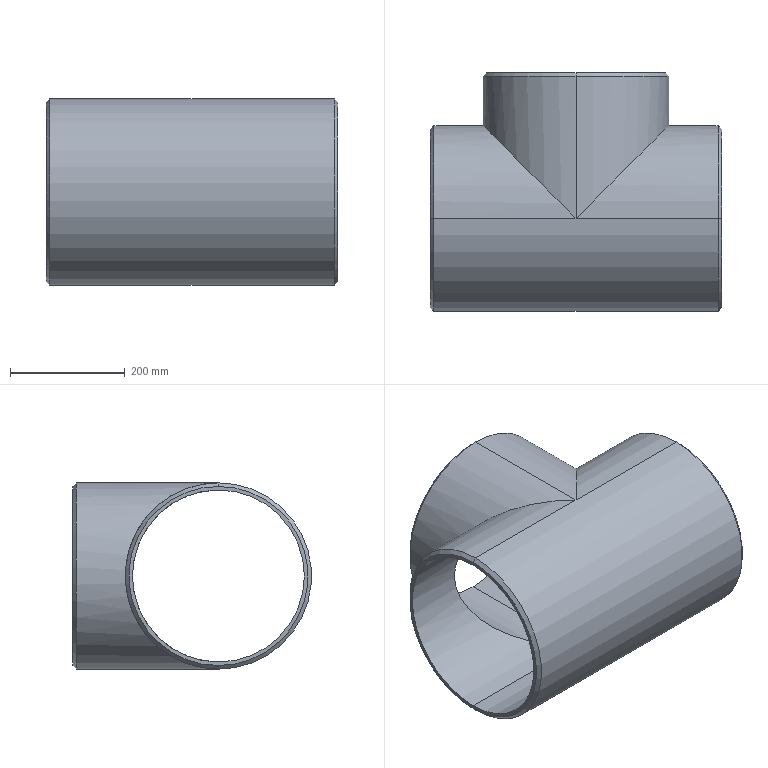Part | NX | features BREP 1 | 1 solid | 19 faces | box 508 x 416.5 x 325 mm | volume 6849380 mm3 | cylinder 10 | cone 6 | plane 3 | commonest cylinder face diameters 300 x5 325 x5
STEP:
#1=CARTESIAN_POINT('',(0.,254.,156.25));
#2=VERTEX_POINT('',#1);
#3=CARTESIAN_POINT('',(0.,254.,-156.25));
#4=VERTEX_POINT('',#3);
#5=CARTESIAN_POINT('',(0.,254.,0.));
#6=DIRECTION('',(0.,1.,0.));
#7=DIRECTION('',(0.,0.,1.));
#8=AXIS2_PLACEMENT_3D('',#5,#6,#7);
#9=CIRCLE('',#8,156.25);
#10=EDGE_CURVE('',#2,#4,#9,.T.);
#11=ORIENTED_EDGE('',*,*,#10,.F.);
#12=CARTESIAN_POINT('',(0.,247.75,162.5));
#13=VERTEX_POINT('',#12);
#14=CARTESIAN_POINT('',(0.,254.,156.25));
#15=DIRECTION('',(0.,-0.7071,0.7071));
#16=VECTOR('',#15,1000.);
#17=LINE('',#14,#16);
#18=EDGE_CURVE('',#13,#2,#17,.F.);
#19=ORIENTED_EDGE('',*,*,#18,.F.);
#20=CARTESIAN_POINT('',(0.,247.75,-162.5));
#21=VERTEX_POINT('',#20);
#22=CARTESIAN_POINT('',(0.,247.75,0.));
#23=DIRECTION('',(0.,-1.,0.));
#24=DIRECTION('',(0.,0.,1.));
#25=AXIS2_PLACEMENT_3D('',#22,#23,#24);
#26=CIRCLE('',#25,162.5);
#27=EDGE_CURVE('',#21,#13,#26,.T.);
#28=ORIENTED_EDGE('',*,*,#27,.F.);
#29=CARTESIAN_POINT('',(0.,254.,-156.25));
#30=DIRECTION('',(0.,-0.7071,-0.7071));
#31=VECTOR('',#30,1000.);
#32=LINE('',#29,#31);
#33=EDGE_CURVE('',#21,#4,#32,.F.);
#34=ORIENTED_EDGE('',*,*,#33,.T.);
#35=EDGE_LOOP('',(#11,#19,#28,#34));
#36=FACE_BOUND('',#35,.T.);
#37=CARTESIAN_POINT('',(0.,254.,0.));
#38=DIRECTION('',(0.,-1.,0.));
#39=DIRECTION('',(0.,0.,1.));
#40=AXIS2_PLACEMENT_3D('',#37,#38,#39);
#41=CONICAL_SURFACE('',#40,156.25,0.7854);
#42=ADVANCED_FACE('',(#36),#41,.T.);
#43=CARTESIAN_POINT('',(254.,0.,-156.25));
#44=VERTEX_POINT('',#43);
#45=CARTESIAN_POINT('',(254.,0.,156.25));
#46=VERTEX_POINT('',#45);
#47=CARTESIAN_POINT('',(254.,0.,0.));
#48=DIRECTION('',(1.,0.,0.));
#49=DIRECTION('',(0.,0.,-1.));
#50=AXIS2_PLACEMENT_3D('',#47,#48,#49);
#51=CIRCLE('',#50,156.25);
#52=EDGE_CURVE('',#44,#46,#51,.T.);
#53=ORIENTED_EDGE('',*,*,#52,.F.);
#54=CARTESIAN_POINT('',(247.75,0.,-162.5));
#55=VERTEX_POINT('',#54);
#56=CARTESIAN_POINT('',(254.,0.,-156.25));
#57=DIRECTION('',(-0.7071,0.,-0.7071));
#58=VECTOR('',#57,1000.);
#59=LINE('',#56,#58);
#60=EDGE_CURVE('',#44,#55,#59,.T.);
#61=ORIENTED_EDGE('',*,*,#60,.T.);
#62=CARTESIAN_POINT('',(247.75,0.,162.5));
#63=VERTEX_POINT('',#62);
#64=CARTESIAN_POINT('',(247.75,0.,0.));
#65=DIRECTION('',(-1.,0.,0.));
#66=DIRECTION('',(0.,0.,-1.));
#67=AXIS2_PLACEMENT_3D('',#64,#65,#66);
#68=CIRCLE('',#67,162.5);
#69=EDGE_CURVE('',#63,#55,#68,.T.);
#70=ORIENTED_EDGE('',*,*,#69,.F.);
#71=CARTESIAN_POINT('',(254.,0.,156.25));
#72=DIRECTION('',(-0.7071,0.,0.7071));
#73=VECTOR('',#72,1000.);
#74=LINE('',#71,#73);
#75=EDGE_CURVE('',#46,#63,#74,.T.);
#76=ORIENTED_EDGE('',*,*,#75,.F.);
#77=EDGE_LOOP('',(#53,#61,#70,#76));
#78=FACE_BOUND('',#77,.T.);
#79=CARTESIAN_POINT('',(254.,0.,0.));
#80=DIRECTION('',(-1.,0.,0.));
#81=DIRECTION('',(0.,0.,-1.));
#82=AXIS2_PLACEMENT_3D('',#79,#80,#81);
#83=CONICAL_SURFACE('',#82,156.25,0.7854);
#84=ADVANCED_FACE('',(#78),#83,.T.);
#85=CARTESIAN_POINT('',(-254.,0.,156.25));
#86=VERTEX_POINT('',#85);
#87=CARTESIAN_POINT('',(-254.,0.,-156.25));
#88=VERTEX_POINT('',#87);
#89=CARTESIAN_POINT('',(-254.,0.,0.));
#90=DIRECTION('',(-1.,0.,0.));
#91=DIRECTION('',(0.,0.,1.));
#92=AXIS2_PLACEMENT_3D('',#89,#90,#91);
#93=CIRCLE('',#92,156.25);
#94=EDGE_CURVE('',#86,#88,#93,.T.);
#95=ORIENTED_EDGE('',*,*,#94,.F.);
#96=CARTESIAN_POINT('',(-247.75,0.,162.5));
#97=VERTEX_POINT('',#96);
#98=CARTESIAN_POINT('',(-247.75,0.,162.5));
#99=DIRECTION('',(0.7071,0.,0.7071));
#100=VECTOR('',#99,1000.);
#101=LINE('',#98,#100);
#102=EDGE_CURVE('',#97,#86,#101,.F.);
#103=ORIENTED_EDGE('',*,*,#102,.F.);
#104=CARTESIAN_POINT('',(-247.75,0.,-162.5));
#105=VERTEX_POINT('',#104);
#106=CARTESIAN_POINT('',(-247.75,0.,0.));
#107=DIRECTION('',(1.,0.,0.));
#108=DIRECTION('',(0.,0.,1.));
#109=AXIS2_PLACEMENT_3D('',#106,#107,#108);
#110=CIRCLE('',#109,162.5);
#111=EDGE_CURVE('',#105,#97,#110,.T.);
#112=ORIENTED_EDGE('',*,*,#111,.F.);
#113=CARTESIAN_POINT('',(-247.75,0.,-162.5));
#114=DIRECTION('',(0.7071,0.,-0.7071));
#115=VECTOR('',#114,1000.);
#116=LINE('',#113,#115);
#117=EDGE_CURVE('',#105,#88,#116,.F.);
#118=ORIENTED_EDGE('',*,*,#117,.T.);
#119=EDGE_LOOP('',(#95,#103,#112,#118));
#120=FACE_BOUND('',#119,.T.);
#121=CARTESIAN_POINT('',(-247.75,0.,0.));
#122=DIRECTION('',(1.,0.,0.));
#123=DIRECTION('',(0.,0.,1.));
#124=AXIS2_PLACEMENT_3D('',#121,#122,#123);
#125=CONICAL_SURFACE('',#124,162.5,0.7854);
#126=ADVANCED_FACE('',(#120),#125,.T.);
#127=CARTESIAN_POINT('',(0.,0.,-150.));
#128=VERTEX_POINT('',#127);
#129=CARTESIAN_POINT('',(0.,0.,150.));
#130=VERTEX_POINT('',#129);
#131=CARTESIAN_POINT('',(0.,0.,-150.));
#132=CARTESIAN_POINT('',(-300.,300.,-150.));
#133=CARTESIAN_POINT('',(-300.,300.,150.));
#134=CARTESIAN_POINT('',(0.,0.,150.));
#135=(BOUNDED_CURVE()B_SPLINE_CURVE(3,(#131,#132,#133,#134),.UNSPECIFIED.,.F.,.F.)B_SPLINE_CURVE_WITH_KNOTS((4,4),(0.,1.),.PIECEWISE_BEZIER_KNOTS.)CURVE()GEOMETRIC_REPRESENTATION_ITEM()RATIONAL_B_SPLINE_CURVE((1.,0.3333,0.3333,1.))REPRESENTATION_ITEM(''));
#136=EDGE_CURVE('',#128,#130,#135,.T.);
#137=ORIENTED_EDGE('',*,*,#136,.F.);
#138=CARTESIAN_POINT('',(0.,254.,-150.));
#139=VERTEX_POINT('',#138);
#140=CARTESIAN_POINT('',(0.,0.,-150.));
#141=DIRECTION('',(0.,1.,0.));
#142=VECTOR('',#141,1000.);
#143=LINE('',#140,#142);
#144=EDGE_CURVE('',#128,#139,#143,.T.);
#145=ORIENTED_EDGE('',*,*,#144,.T.);
#146=CARTESIAN_POINT('',(0.,254.,150.));
#147=VERTEX_POINT('',#146);
#148=CARTESIAN_POINT('',(0.,254.,0.));
#149=DIRECTION('',(0.,1.,0.));
#150=DIRECTION('',(0.,0.,1.));
#151=AXIS2_PLACEMENT_3D('',#148,#149,#150);
#152=CIRCLE('',#151,150.);
#153=EDGE_CURVE('',#139,#147,#152,.T.);
#154=ORIENTED_EDGE('',*,*,#153,.T.);
#155=CARTESIAN_POINT('',(0.,0.,150.));
#156=DIRECTION('',(0.,1.,0.));
#157=VECTOR('',#156,1000.);
#158=LINE('',#155,#157);
#159=EDGE_CURVE('',#130,#147,#158,.T.);
#160=ORIENTED_EDGE('',*,*,#159,.F.);
#161=EDGE_LOOP('',(#137,#145,#154,#160));
#162=FACE_BOUND('',#161,.T.);
#163=CARTESIAN_POINT('',(0.,0.,0.));
#164=DIRECTION('',(0.,1.,0.));
#165=DIRECTION('',(0.,0.,-1.));
#166=AXIS2_PLACEMENT_3D('',#163,#164,#165);
#167=CYLINDRICAL_SURFACE('',#166,150.);
#168=ADVANCED_FACE('',(#162),#167,.F.);
#169=CARTESIAN_POINT('',(254.,0.,-150.));
#170=VERTEX_POINT('',#169);
#171=CARTESIAN_POINT('',(254.,0.,150.));
#172=VERTEX_POINT('',#171);
#173=CARTESIAN_POINT('',(254.,0.,0.));
#174=DIRECTION('',(-1.,0.,0.));
#175=DIRECTION('',(0.,0.,1.));
#176=AXIS2_PLACEMENT_3D('',#173,#174,#175);
#177=CIRCLE('',#176,150.);
#178=EDGE_CURVE('',#170,#172,#177,.T.);
#179=ORIENTED_EDGE('',*,*,#178,.F.);
#180=CARTESIAN_POINT('',(254.,0.,-150.));
#181=DIRECTION('',(-1.,0.,0.));
#182=VECTOR('',#181,1000.);
#183=LINE('',#180,#182);
#184=EDGE_CURVE('',#170,#128,#183,.T.);
#185=ORIENTED_EDGE('',*,*,#184,.T.);
#186=CARTESIAN_POINT('',(-254.,0.,-150.));
#187=VERTEX_POINT('',#186);
#188=CARTESIAN_POINT('',(254.,0.,-150.));
#189=DIRECTION('',(-1.,0.,0.));
#190=VECTOR('',#189,1000.);
#191=LINE('',#188,#190);
#192=EDGE_CURVE('',#128,#187,#191,.T.);
#193=ORIENTED_EDGE('',*,*,#192,.T.);
#194=CARTESIAN_POINT('',(-254.,0.,150.));
#195=VERTEX_POINT('',#194);
#196=CARTESIAN_POINT('',(-254.,0.,0.));
#197=DIRECTION('',(-1.,0.,0.));
#198=DIRECTION('',(0.,0.,1.));
#199=AXIS2_PLACEMENT_3D('',#196,#197,#198);
#200=CIRCLE('',#199,150.);
#201=EDGE_CURVE('',#187,#195,#200,.T.);
#202=ORIENTED_EDGE('',*,*,#201,.T.);
#203=CARTESIAN_POINT('',(254.,0.,150.));
#204=DIRECTION('',(-1.,0.,0.));
#205=VECTOR('',#204,1000.);
#206=LINE('',#203,#205);
#207=EDGE_CURVE('',#130,#195,#206,.T.);
#208=ORIENTED_EDGE('',*,*,#207,.F.);
#209=CARTESIAN_POINT('',(254.,0.,150.));
#210=DIRECTION('',(-1.,0.,0.));
#211=VECTOR('',#210,1000.);
#212=LINE('',#209,#211);
#213=EDGE_CURVE('',#172,#130,#212,.T.);
#214=ORIENTED_EDGE('',*,*,#213,.F.);
#215=EDGE_LOOP('',(#179,#185,#193,#202,#208,#214));
#216=FACE_BOUND('',#215,.T.);
#217=CARTESIAN_POINT('',(254.,0.,0.));
#218=DIRECTION('',(-1.,0.,0.));
#219=DIRECTION('',(0.,0.,-1.));
#220=AXIS2_PLACEMENT_3D('',#217,#218,#219);
#221=CYLINDRICAL_SURFACE('',#220,150.);
#222=ADVANCED_FACE('',(#216),#221,.F.);
#223=ORIENTED_EDGE('',*,*,#184,.F.);
#224=CARTESIAN_POINT('',(254.,0.,0.));
#225=DIRECTION('',(-1.,0.,0.));
#226=DIRECTION('',(0.,0.,1.));
#227=AXIS2_PLACEMENT_3D('',#224,#225,#226);
#228=CIRCLE('',#227,150.);
#229=EDGE_CURVE('',#172,#170,#228,.T.);
#230=ORIENTED_EDGE('',*,*,#229,.F.);
#231=ORIENTED_EDGE('',*,*,#213,.T.);
#232=CARTESIAN_POINT('',(0.,0.,150.));
#233=CARTESIAN_POINT('',(300.,300.,150.));
#234=CARTESIAN_POINT('',(300.,300.,-150.));
#235=CARTESIAN_POINT('',(0.,0.,-150.));
#236=(BOUNDED_CURVE()B_SPLINE_CURVE(3,(#232,#233,#234,#235),.UNSPECIFIED.,.F.,.F.)B_SPLINE_CURVE_WITH_KNOTS((4,4),(0.,1.),.PIECEWISE_BEZIER_KNOTS.)CURVE()GEOMETRIC_REPRESENTATION_ITEM()RATIONAL_B_SPLINE_CURVE((1.,0.3333,0.3333,1.))REPRESENTATION_ITEM(''));
#237=EDGE_CURVE('',#130,#128,#236,.T.);
#238=ORIENTED_EDGE('',*,*,#237,.T.);
#239=EDGE_LOOP('',(#223,#230,#231,#238));
#240=FACE_BOUND('',#239,.T.);
#241=CARTESIAN_POINT('',(254.,0.,0.));
#242=DIRECTION('',(-1.,0.,0.));
#243=DIRECTION('',(0.,0.,-1.));
#244=AXIS2_PLACEMENT_3D('',#241,#242,#243);
#245=CYLINDRICAL_SURFACE('',#244,150.);
#246=ADVANCED_FACE('',(#240),#245,.F.);
#247=ORIENTED_EDGE('',*,*,#27,.T.);
#248=CARTESIAN_POINT('',(0.,0.,162.5));
#249=VERTEX_POINT('',#248);
#250=CARTESIAN_POINT('',(0.,254.,162.5));
#251=DIRECTION('',(0.,-1.,0.));
#252=VECTOR('',#251,1000.);
#253=LINE('',#250,#252);
#254=EDGE_CURVE('',#249,#13,#253,.F.);
#255=ORIENTED_EDGE('',*,*,#254,.F.);
#256=CARTESIAN_POINT('',(0.,0.,-162.5));
#257=VERTEX_POINT('',#256);
#258=CARTESIAN_POINT('',(0.,0.,162.5));
#259=CARTESIAN_POINT('',(325.,325.,162.5));
#260=CARTESIAN_POINT('',(325.,325.,-162.5));
#261=CARTESIAN_POINT('',(0.,0.,-162.5));
#262=(BOUNDED_CURVE()B_SPLINE_CURVE(3,(#258,#259,#260,#261),.UNSPECIFIED.,.F.,.F.)B_SPLINE_CURVE_WITH_KNOTS((4,4),(0.,1.),.PIECEWISE_BEZIER_KNOTS.)CURVE()GEOMETRIC_REPRESENTATION_ITEM()RATIONAL_B_SPLINE_CURVE((1.,0.3333,0.3333,1.))REPRESENTATION_ITEM(''));
#263=EDGE_CURVE('',#249,#257,#262,.T.);
#264=ORIENTED_EDGE('',*,*,#263,.T.);
#265=CARTESIAN_POINT('',(0.,254.,-162.5));
#266=DIRECTION('',(0.,-1.,0.));
#267=VECTOR('',#266,1000.);
#268=LINE('',#265,#267);
#269=EDGE_CURVE('',#257,#21,#268,.F.);
#270=ORIENTED_EDGE('',*,*,#269,.T.);
#271=EDGE_LOOP('',(#247,#255,#264,#270));
#272=FACE_BOUND('',#271,.T.);
#273=CARTESIAN_POINT('',(0.,254.,0.));
#274=DIRECTION('',(0.,-1.,0.));
#275=DIRECTION('',(0.,0.,1.));
#276=AXIS2_PLACEMENT_3D('',#273,#274,#275);
#277=CYLINDRICAL_SURFACE('',#276,162.5);
#278=ADVANCED_FACE('',(#272),#277,.T.);
#279=ORIENTED_EDGE('',*,*,#69,.T.);
#280=CARTESIAN_POINT('',(254.,0.,-162.5));
#281=DIRECTION('',(-1.,0.,0.));
#282=VECTOR('',#281,1000.);
#283=LINE('',#280,#282);
#284=EDGE_CURVE('',#55,#257,#283,.T.);
#285=ORIENTED_EDGE('',*,*,#284,.T.);
#286=ORIENTED_EDGE('',*,*,#263,.F.);
#287=CARTESIAN_POINT('',(254.,0.,162.5));
#288=DIRECTION('',(-1.,0.,0.));
#289=VECTOR('',#288,1000.);
#290=LINE('',#287,#289);
#291=EDGE_CURVE('',#63,#249,#290,.T.);
#292=ORIENTED_EDGE('',*,*,#291,.F.);
#293=EDGE_LOOP('',(#279,#285,#286,#292));
#294=FACE_BOUND('',#293,.T.);
#295=CARTESIAN_POINT('',(254.,0.,0.));
#296=DIRECTION('',(-1.,0.,0.));
#297=DIRECTION('',(0.,0.,-1.));
#298=AXIS2_PLACEMENT_3D('',#295,#296,#297);
#299=CYLINDRICAL_SURFACE('',#298,162.5);
#300=ADVANCED_FACE('',(#294),#299,.T.);
#301=CARTESIAN_POINT('',(0.,0.,-162.5));
#302=CARTESIAN_POINT('',(-325.,325.,-162.5));
#303=CARTESIAN_POINT('',(-325.,325.,162.5));
#304=CARTESIAN_POINT('',(0.,0.,162.5));
#305=(BOUNDED_CURVE()B_SPLINE_CURVE(3,(#301,#302,#303,#304),.UNSPECIFIED.,.F.,.F.)B_SPLINE_CURVE_WITH_KNOTS((4,4),(0.,1.),.PIECEWISE_BEZIER_KNOTS.)CURVE()GEOMETRIC_REPRESENTATION_ITEM()RATIONAL_B_SPLINE_CURVE((1.,0.3333,0.3333,1.))REPRESENTATION_ITEM(''));
#306=EDGE_CURVE('',#257,#249,#305,.T.);
#307=ORIENTED_EDGE('',*,*,#306,.F.);
#308=CARTESIAN_POINT('',(254.,0.,-162.5));
#309=DIRECTION('',(-1.,0.,0.));
#310=VECTOR('',#309,1000.);
#311=LINE('',#308,#310);
#312=EDGE_CURVE('',#257,#105,#311,.T.);
#313=ORIENTED_EDGE('',*,*,#312,.T.);
#314=ORIENTED_EDGE('',*,*,#111,.T.);
#315=CARTESIAN_POINT('',(254.,0.,162.5));
#316=DIRECTION('',(-1.,0.,0.));
#317=VECTOR('',#316,1000.);
#318=LINE('',#315,#317);
#319=EDGE_CURVE('',#249,#97,#318,.T.);
#320=ORIENTED_EDGE('',*,*,#319,.F.);
#321=EDGE_LOOP('',(#307,#313,#314,#320));
#322=FACE_BOUND('',#321,.T.);
#323=CARTESIAN_POINT('',(254.,0.,0.));
#324=DIRECTION('',(-1.,0.,0.));
#325=DIRECTION('',(0.,0.,-1.));
#326=AXIS2_PLACEMENT_3D('',#323,#324,#325);
#327=CYLINDRICAL_SURFACE('',#326,162.5);
#328=ADVANCED_FACE('',(#322),#327,.T.);
#329=ORIENTED_EDGE('',*,*,#284,.F.);
#330=CARTESIAN_POINT('',(247.75,0.,0.));
#331=DIRECTION('',(-1.,0.,0.));
#332=DIRECTION('',(0.,0.,-1.));
#333=AXIS2_PLACEMENT_3D('',#330,#331,#332);
#334=CIRCLE('',#333,162.5);
#335=EDGE_CURVE('',#55,#63,#334,.T.);
#336=ORIENTED_EDGE('',*,*,#335,.T.);
#337=ORIENTED_EDGE('',*,*,#291,.T.);
#338=ORIENTED_EDGE('',*,*,#319,.T.);
#339=CARTESIAN_POINT('',(-247.75,0.,0.));
#340=DIRECTION('',(1.,0.,0.));
#341=DIRECTION('',(0.,0.,1.));
#342=AXIS2_PLACEMENT_3D('',#339,#340,#341);
#343=CIRCLE('',#342,162.5);
#344=EDGE_CURVE('',#97,#105,#343,.T.);
#345=ORIENTED_EDGE('',*,*,#344,.T.);
#346=ORIENTED_EDGE('',*,*,#312,.F.);
#347=EDGE_LOOP('',(#329,#336,#337,#338,#345,#346));
#348=FACE_BOUND('',#347,.T.);
#349=CARTESIAN_POINT('',(254.,0.,0.));
#350=DIRECTION('',(-1.,0.,0.));
#351=DIRECTION('',(0.,0.,-1.));
#352=AXIS2_PLACEMENT_3D('',#349,#350,#351);
#353=CYLINDRICAL_SURFACE('',#352,162.5);
#354=ADVANCED_FACE('',(#348),#353,.T.);
#355=CARTESIAN_POINT('',(254.,0.,0.));
#356=DIRECTION('',(1.,0.,0.));
#357=DIRECTION('',(0.,0.,-1.));
#358=AXIS2_PLACEMENT_3D('',#355,#356,#357);
#359=CIRCLE('',#358,156.25);
#360=EDGE_CURVE('',#46,#44,#359,.T.);
#361=ORIENTED_EDGE('',*,*,#360,.T.);
#362=ORIENTED_EDGE('',*,*,#52,.T.);
#363=EDGE_LOOP('',(#361,#362));
#364=FACE_BOUND('',#363,.T.);
#365=ORIENTED_EDGE('',*,*,#229,.T.);
#366=ORIENTED_EDGE('',*,*,#178,.T.);
#367=EDGE_LOOP('',(#365,#366));
#368=FACE_BOUND('',#367,.T.);
#369=CARTESIAN_POINT('',(254.,0.,0.));
#370=DIRECTION('',(1.,0.,0.));
#371=DIRECTION('',(0.,0.,1.));
#372=AXIS2_PLACEMENT_3D('',#369,#370,#371);
#373=PLANE('',#372);
#374=ADVANCED_FACE('',(#364,#368),#373,.T.);
#375=ORIENTED_EDGE('',*,*,#254,.T.);
#376=CARTESIAN_POINT('',(0.,247.75,0.));
#377=DIRECTION('',(0.,-1.,0.));
#378=DIRECTION('',(0.,0.,1.));
#379=AXIS2_PLACEMENT_3D('',#376,#377,#378);
#380=CIRCLE('',#379,162.5);
#381=EDGE_CURVE('',#13,#21,#380,.T.);
#382=ORIENTED_EDGE('',*,*,#381,.T.);
#383=ORIENTED_EDGE('',*,*,#269,.F.);
#384=ORIENTED_EDGE('',*,*,#306,.T.);
#385=EDGE_LOOP('',(#375,#382,#383,#384));
#386=FACE_BOUND('',#385,.T.);
#387=CARTESIAN_POINT('',(0.,254.,0.));
#388=DIRECTION('',(0.,-1.,0.));
#389=DIRECTION('',(0.,0.,1.));
#390=AXIS2_PLACEMENT_3D('',#387,#388,#389);
#391=CYLINDRICAL_SURFACE('',#390,162.5);
#392=ADVANCED_FACE('',(#386),#391,.T.);
#393=CARTESIAN_POINT('',(0.,254.,0.));
#394=DIRECTION('',(0.,1.,0.));
#395=DIRECTION('',(0.,0.,1.));
#396=AXIS2_PLACEMENT_3D('',#393,#394,#395);
#397=CIRCLE('',#396,156.25);
#398=EDGE_CURVE('',#4,#2,#397,.T.);
#399=ORIENTED_EDGE('',*,*,#398,.T.);
#400=ORIENTED_EDGE('',*,*,#10,.T.);
#401=EDGE_LOOP('',(#399,#400));
#402=FACE_BOUND('',#401,.T.);
#403=CARTESIAN_POINT('',(0.,254.,0.));
#404=DIRECTION('',(0.,1.,0.));
#405=DIRECTION('',(0.,0.,1.));
#406=AXIS2_PLACEMENT_3D('',#403,#404,#405);
#407=CIRCLE('',#406,150.);
#408=EDGE_CURVE('',#147,#139,#407,.T.);
#409=ORIENTED_EDGE('',*,*,#408,.F.);
#410=ORIENTED_EDGE('',*,*,#153,.F.);
#411=EDGE_LOOP('',(#409,#410));
#412=FACE_BOUND('',#411,.T.);
#413=CARTESIAN_POINT('',(0.,254.,0.));
#414=DIRECTION('',(0.,1.,0.));
#415=DIRECTION('',(0.,0.,-1.));
#416=AXIS2_PLACEMENT_3D('',#413,#414,#415);
#417=PLANE('',#416);
#418=ADVANCED_FACE('',(#402,#412),#417,.T.);
#419=CARTESIAN_POINT('',(-254.,0.,0.));
#420=DIRECTION('',(-1.,0.,0.));
#421=DIRECTION('',(0.,0.,1.));
#422=AXIS2_PLACEMENT_3D('',#419,#420,#421);
#423=CIRCLE('',#422,156.25);
#424=EDGE_CURVE('',#88,#86,#423,.T.);
#425=ORIENTED_EDGE('',*,*,#424,.T.);
#426=ORIENTED_EDGE('',*,*,#94,.T.);
#427=EDGE_LOOP('',(#425,#426));
#428=FACE_BOUND('',#427,.T.);
#429=CARTESIAN_POINT('',(-254.,0.,0.));
#430=DIRECTION('',(-1.,0.,0.));
#431=DIRECTION('',(0.,0.,1.));
#432=AXIS2_PLACEMENT_3D('',#429,#430,#431);
#433=CIRCLE('',#432,150.);
#434=EDGE_CURVE('',#195,#187,#433,.T.);
#435=ORIENTED_EDGE('',*,*,#434,.F.);
#436=ORIENTED_EDGE('',*,*,#201,.F.);
#437=EDGE_LOOP('',(#435,#436));
#438=FACE_BOUND('',#437,.T.);
#439=CARTESIAN_POINT('',(-254.,0.,0.));
#440=DIRECTION('',(-1.,0.,0.));
#441=DIRECTION('',(0.,0.,1.));
#442=AXIS2_PLACEMENT_3D('',#439,#440,#441);
#443=PLANE('',#442);
#444=ADVANCED_FACE('',(#428,#438),#443,.T.);
#445=ORIENTED_EDGE('',*,*,#192,.F.);
#446=ORIENTED_EDGE('',*,*,#136,.T.);
#447=ORIENTED_EDGE('',*,*,#207,.T.);
#448=ORIENTED_EDGE('',*,*,#434,.T.);
#449=EDGE_LOOP('',(#445,#446,#447,#448));
#450=FACE_BOUND('',#449,.T.);
#451=CARTESIAN_POINT('',(254.,0.,0.));
#452=DIRECTION('',(-1.,0.,0.));
#453=DIRECTION('',(0.,0.,-1.));
#454=AXIS2_PLACEMENT_3D('',#451,#452,#453);
#455=CYLINDRICAL_SURFACE('',#454,150.);
#456=ADVANCED_FACE('',(#450),#455,.F.);
#457=ORIENTED_EDGE('',*,*,#144,.F.);
#458=ORIENTED_EDGE('',*,*,#237,.F.);
#459=ORIENTED_EDGE('',*,*,#159,.T.);
#460=ORIENTED_EDGE('',*,*,#408,.T.);
#461=EDGE_LOOP('',(#457,#458,#459,#460));
#462=FACE_BOUND('',#461,.T.);
#463=CARTESIAN_POINT('',(0.,0.,0.));
#464=DIRECTION('',(0.,1.,0.));
#465=DIRECTION('',(0.,0.,-1.));
#466=AXIS2_PLACEMENT_3D('',#463,#464,#465);
#467=CYLINDRICAL_SURFACE('',#466,150.);
#468=ADVANCED_FACE('',(#462),#467,.F.);
#469=ORIENTED_EDGE('',*,*,#102,.T.);
#470=ORIENTED_EDGE('',*,*,#424,.F.);
#471=ORIENTED_EDGE('',*,*,#117,.F.);
#472=ORIENTED_EDGE('',*,*,#344,.F.);
#473=EDGE_LOOP('',(#469,#470,#471,#472));
#474=FACE_BOUND('',#473,.T.);
#475=CARTESIAN_POINT('',(-247.75,0.,0.));
#476=DIRECTION('',(1.,0.,0.));
#477=DIRECTION('',(0.,0.,1.));
#478=AXIS2_PLACEMENT_3D('',#475,#476,#477);
#479=CONICAL_SURFACE('',#478,162.5,0.7854);
#480=ADVANCED_FACE('',(#474),#479,.T.);
#481=ORIENTED_EDGE('',*,*,#60,.F.);
#482=ORIENTED_EDGE('',*,*,#360,.F.);
#483=ORIENTED_EDGE('',*,*,#75,.T.);
#484=ORIENTED_EDGE('',*,*,#335,.F.);
#485=EDGE_LOOP('',(#481,#482,#483,#484));
#486=FACE_BOUND('',#485,.T.);
#487=CARTESIAN_POINT('',(254.,0.,0.));
#488=DIRECTION('',(-1.,0.,0.));
#489=DIRECTION('',(0.,0.,-1.));
#490=AXIS2_PLACEMENT_3D('',#487,#488,#489);
#491=CONICAL_SURFACE('',#490,156.25,0.7854);
#492=ADVANCED_FACE('',(#486),#491,.T.);
#493=ORIENTED_EDGE('',*,*,#18,.T.);
#494=ORIENTED_EDGE('',*,*,#398,.F.);
#495=ORIENTED_EDGE('',*,*,#33,.F.);
#496=ORIENTED_EDGE('',*,*,#381,.F.);
#497=EDGE_LOOP('',(#493,#494,#495,#496));
#498=FACE_BOUND('',#497,.T.);
#499=CARTESIAN_POINT('',(0.,254.,0.));
#500=DIRECTION('',(0.,-1.,0.));
#501=DIRECTION('',(0.,0.,1.));
#502=AXIS2_PLACEMENT_3D('',#499,#500,#501);
#503=CONICAL_SURFACE('',#502,156.25,0.7854);
#504=ADVANCED_FACE('',(#498),#503,.T.);
#505=CLOSED_SHELL('',(#42,#84,#126,#168,#222,#246,#278,#300,#328,#354,#374,#392,#418,#444,#456,#468,#480,#492,#504));
#506=MANIFOLD_SOLID_BREP('',#505);
#507=(LENGTH_UNIT()NAMED_UNIT(*)SI_UNIT(.MILLI.,.METRE.));
#508=UNCERTAINTY_MEASURE_WITH_UNIT(LENGTH_MEASURE(0.00001),#507,'','');
#509=(NAMED_UNIT(*)PLANE_ANGLE_UNIT()SI_UNIT($,.RADIAN.));
#510=(NAMED_UNIT(*)SI_UNIT($,.STERADIAN.)SOLID_ANGLE_UNIT());
#511=(GEOMETRIC_REPRESENTATION_CONTEXT(3)GLOBAL_UNCERTAINTY_ASSIGNED_CONTEXT((#508))GLOBAL_UNIT_ASSIGNED_CONTEXT((#507,#509,#510))REPRESENTATION_CONTEXT('',''));
#512=ADVANCED_BREP_SHAPE_REPRESENTATION('',(#506),#511);